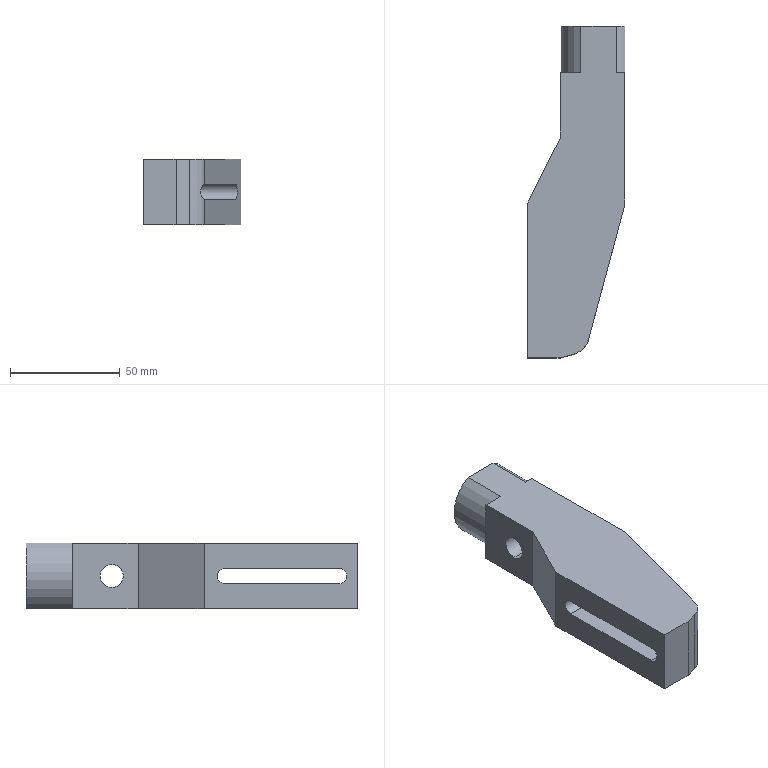Part | STEP file | 1 solid | 23 faces | box 44.5 x 151 x 30 mm | volume 132729 mm3 | plane 15 | cylinder 8 | commonest cylinder face diameters 34 x3 7 x2 10.5 x2 20 x1